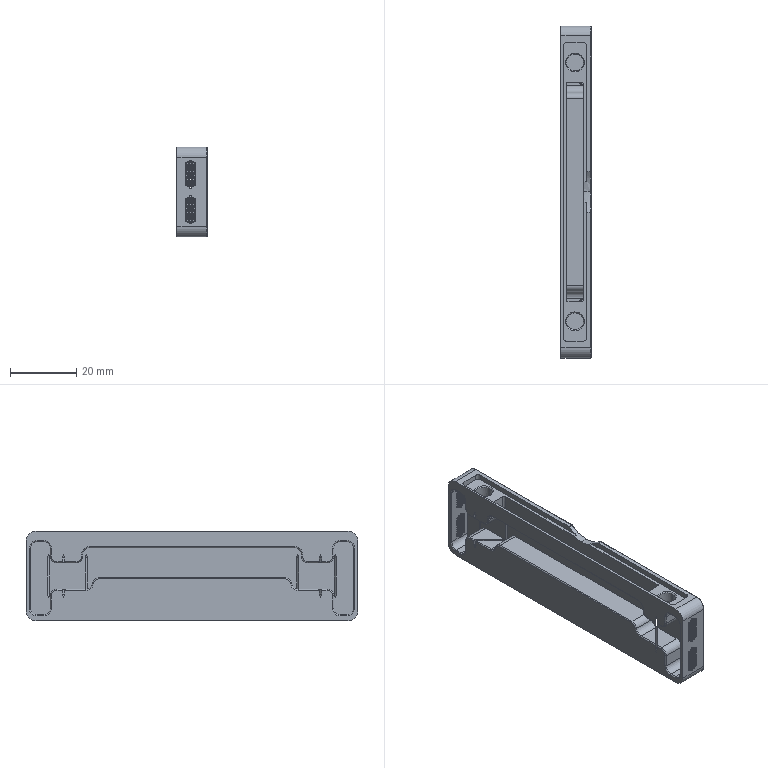Part | SolidWorks | features ICE 3, MoveFace 3, BaseBody 1, MirrorPattern 1 | 1 solid | 724 faces | box 9.09 x 100 x 27 mm | volume 14377 mm3 | cylinder 463 | plane 151 | spline 106 | cone 4 | commonest cylinder face diameters 0.5 x392 4 x24 0.6 x22 0.4 x7 1 x4 2 x4